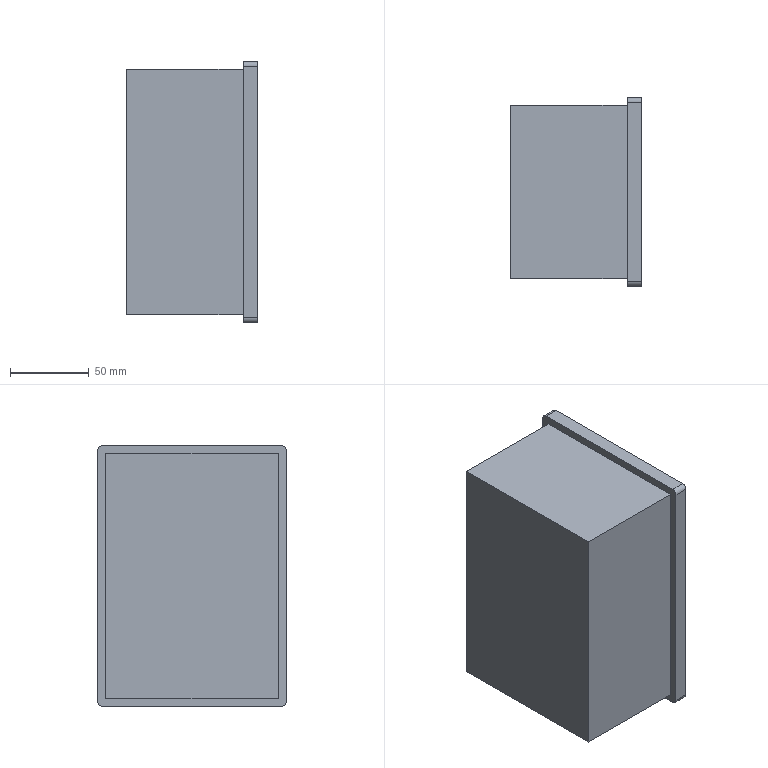Part | STEP file | TCN-002 Tension cont roller^Tension control panel | 1 solid | 306 faces | box 83 x 120 x 166 mm | volume 1448834 mm3 | plane 228 | spline 57 | cylinder 21 | commonest cylinder face diameters 6 x12 5 x4 1.067 x1 1.19 x1 1.798 x1 5.008 x1